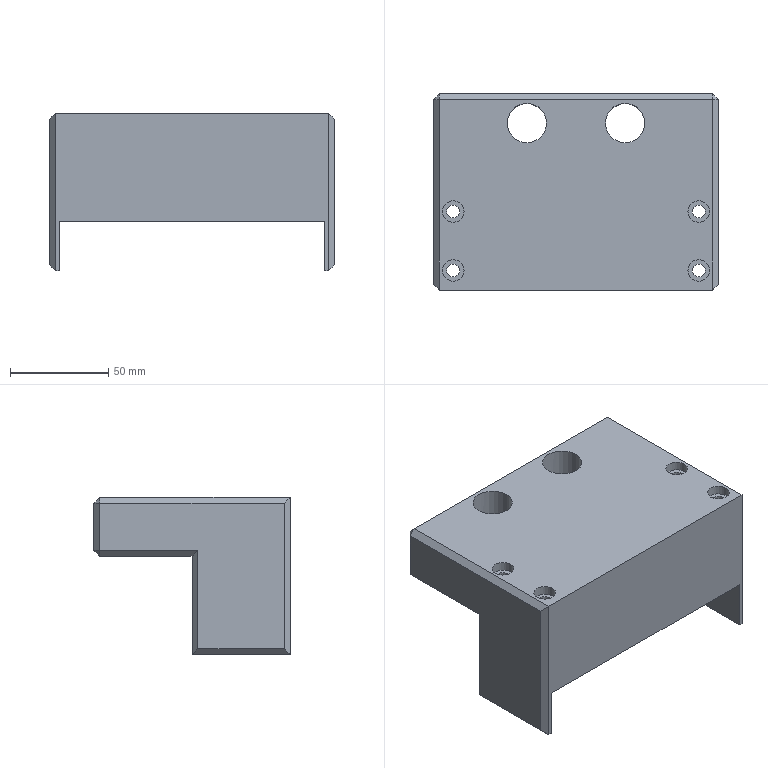NC program | NX | posted with a generic post | part box 145 x 100 x 80 mm
Lines 551 to 2025 of 2025, first 1325 of 1469 lines:
(ZLEVEL_PROFILE_1_COPY_1_COPY_COPY_1_COPY_COPY_COPY_COPY , TOOL : D8A45)
N1076 T06 M6
N1078 G54
N1080 G17 G0 G90 X-70.793 Y41.932 B0. C0. S7500 M3
N1082 G43 Z30. H6
N1084 Z-2.5
N1086 G94 G1 Z-3.5 F1000.
N1088 X-70.197 Y40.9
N1090 G3 X-69.504 Y40.5 R0.8
N1092 G1 X69.504
N1094 G2 X73. Y37.001 R3.504
N1096 G1 Y12.999
N1098 G2 X69.504 Y9.5 R3.498
N1100 G1 X-69.504
N1102 G2 X-73. Y12.999 R3.497
N1104 G1 Y37.001
N1106 G2 X-69.504 Y40.5 R3.504
N1108 G3 X-68.812 Y40.902 R0.8
N1110 G1 X-68.124 Y42.1
N1112 Z-2.5
N1114 G0 Z30.
(ZLEVEL_PROFILE_1_COPY_1_COPY_COPY_1_COPY_COPY_COPY_COPY_COPY , TOOL : D8A45)
N1116 X74.991 Y7.571
N1118 Z-52.5
N1120 G1 Z-53.5
N1122 X73.773 Y7.898
N1124 G3 X73. Y7.691 R0.8
N1126 G1 Y-37.002
N1128 Y-40.021
N1130 G2 X69.501 Y-43.5 R3.504
N1132 G1 X67.499
N1134 G2 X64. Y-40. R3.499
N1136 G1 Y-18.5
N1138 X-64.
N1140 Y-40.
N1142 G2 X-67.499 Y-43.5 R3.499
N1144 G1 X-69.501
N1146 G2 X-73. Y-40.021 R3.504
N1148 G1 Y-37.002
N1150 Y7.691
N1152 G3 X-73.773 Y7.898 R0.8
N1154 G1 X-74.991 Y7.571
N1156 Z-52.5
N1158 G0 Z30.
(ZLEVEL_PROFILE_1_COPY_1_COPY_COPY_1_COPY_COPY_COPY_COPY_COPY_COPY , TOOL : D8A45)
N1160 X-23.384 Y28.089
N1162 Z0.647
N1164 G1 Z-0.353
N1166 X-24.306 Y29.685
N1168 G3 X-24.999 Y30.085 R0.8
N1170 X-30.086 Y24.998 R5.087
N1172 X-24.999 Y30.085 R-5.087
N1174 G1 X-25.197 Y30.08 Z-0.357
N1176 X-25.395 Y30.065 Z-0.36
N1178 X-25.592 Y30.049 Z-0.364
N1180 X-25.69 Y30.031 Z-0.365
N1182 X-25.787 Y30.012 Z-0.367
N1184 X-26.175 Y29.935 Z-0.374
N1186 X-26.364 Y29.876 Z-0.377
N1188 X-26.552 Y29.815 Z-0.381
N1190 X-26.74 Y29.754 Z-0.384
N1192 X-26.831 Y29.715 Z-0.386
N1194 X-26.921 Y29.674 Z-0.388
N1196 X-27.278 Y29.509 Z-0.395
N1198 X-27.448 Y29.409 Z-0.398
N1200 X-27.616 Y29.306 Z-0.402
N1202 X-27.783 Y29.203 Z-0.405
N1204 X-27.941 Y29.084 Z-0.409
N1206 X-28.248 Y28.841 Z-0.416
N1208 X-28.389 Y28.704 Z-0.419
N1210 X-28.528 Y28.565 Z-0.423
N1212 X-28.666 Y28.427 Z-0.426
N1214 X-28.791 Y28.276 Z-0.429
N1216 X-29.032 Y27.969 Z-0.436
N1218 X-29.14 Y27.806 Z-0.44
N1220 X-29.241 Y27.639 Z-0.443
N1222 X-29.342 Y27.472 Z-0.447
N1224 X-29.43 Y27.298 Z-0.45
N1226 X-29.591 Y26.944 Z-0.457
N1228 X-29.659 Y26.762 Z-0.461
N1230 X-29.718 Y26.577 Z-0.464
N1232 X-29.777 Y26.392 Z-0.468
N1234 X-29.823 Y26.203 Z-0.471
N1236 X-29.896 Y25.822 Z-0.478
N1238 X-29.92 Y25.631 Z-0.481
N1240 X-29.934 Y25.437 Z-0.485
N1242 X-29.948 Y25.245 Z-0.488
N1244 X-29.95 Y25.051 Z-0.492
N1246 X-29.932 Y24.666 Z-0.499
N1248 X-29.913 Y24.474 Z-0.502
N1250 X-29.881 Y24.284 Z-0.506
N1252 X-29.849 Y24.094 Z-0.509
N1254 X-29.808 Y23.906 Z-0.513
N1256 X-29.7 Y23.537 Z-0.519
N1258 X-29.638 Y23.356 Z-0.523
N1260 X-29.563 Y23.179 Z-0.526
N1262 X-29.487 Y23.003 Z-0.53
N1264 X-29.405 Y22.83 Z-0.533
N1266 X-29.214 Y22.498 Z-0.54
N1268 X-29.113 Y22.336 Z-0.544
N1270 X-28.999 Y22.183 Z-0.547
N1272 X-28.885 Y22.03 Z-0.551
N1274 X-28.767 Y21.88 Z-0.554
N1276 X-28.504 Y21.604 Z-0.561
N1278 X-28.37 Y21.469 Z-0.564
N1280 X-28.223 Y21.348 Z-0.568
N1282 X-28.077 Y21.226 Z-0.571
N1284 X-27.929 Y21.108 Z-0.575
N1286 X-27.61 Y20.902 Z-0.582
N1288 X-27.449 Y20.801 Z-0.585
N1290 X-27.279 Y20.718 Z-0.589
N1292 X-27.109 Y20.635 Z-0.592
N1294 X-26.939 Y20.553 Z-0.596
N1296 X-26.582 Y20.428 Z-0.603
N1298 X-26.493 Y20.397 Z-0.604
N1300 X-26.404 Y20.367 Z-0.606
N1302 X-26.219 Y20.326 Z-0.61
N1304 X-26.035 Y20.285 Z-0.613
N1306 X-25.851 Y20.245 Z-0.616
N1308 X-25.477 Y20.207 Z-0.623
N1310 X-25.29 Y20.188 Z-0.627
N1312 X-25.196 Y20.189 Z-0.629
N1314 X-25.102 Y20.191 Z-0.63
N1316 X-24.727 Y20.198 Z-0.637
N1318 X-24.541 Y20.222 Z-0.641
N1320 X-24.356 Y20.248 Z-0.644
N1322 X-24.171 Y20.273 Z-0.648
N1324 X-23.989 Y20.318 Z-0.651
N1326 X-23.628 Y20.413 Z-0.658
N1328 X-23.453 Y20.478 Z-0.661
N1330 X-23.28 Y20.546 Z-0.665
N1332 X-23.106 Y20.614 Z-0.668
N1334 X-22.94 Y20.699 Z-0.672
N1336 X-22.613 Y20.874 Z-0.679
N1338 X-22.458 Y20.977 Z-0.682
N1340 X-22.306 Y21.083 Z-0.686
N1342 X-22.154 Y21.19 Z-0.689
N1344 X-22.012 Y21.309 Z-0.693
N1346 X-21.737 Y21.556 Z-0.7
N1348 X-21.61 Y21.69 Z-0.703
N1350 X-21.486 Y21.828 Z-0.706
N1352 G3 X-24.999 Y29.734 R4.734
N1354 G1 X-25.197 Y29.726 Z-0.71
N1356 X-25.394 Y29.711 Z-0.713
N1358 X-25.592 Y29.692 Z-0.717
N1360 X-25.786 Y29.653 Z-0.72
N1362 X-25.98 Y29.615 Z-0.724
N1364 X-26.172 Y29.569 Z-0.727
N1366 X-26.548 Y29.447 Z-0.734
N1368 X-26.731 Y29.375 Z-0.738
N1370 X-26.911 Y29.292 Z-0.741
N1372 X-27.089 Y29.21 Z-0.745
N1374 X-27.261 Y29.113 Z-0.748
N1376 X-27.596 Y28.907 Z-0.755
N1378 X-27.752 Y28.788 Z-0.758
N1380 X-27.906 Y28.666 Z-0.762
N1382 X-27.983 Y28.605 Z-0.764
N1384 X-28.058 Y28.543 Z-0.765
N1386 X-28.197 Y28.404 Z-0.769
N1388 X-28.335 Y28.265 Z-0.772
N1390 X-28.47 Y28.123 Z-0.776
N1392 X-28.711 Y27.815 Z-0.783
N1394 X-28.824 Y27.657 Z-0.786
N1396 X-28.925 Y27.49 Z-0.79
N1398 X-29.026 Y27.323 Z-0.793
N1400 X-29.117 Y27.151 Z-0.797
N1402 X-29.278 Y26.797 Z-0.803
N1404 X-29.343 Y26.614 Z-0.807
N1406 X-29.402 Y26.429 Z-0.81
N1408 X-29.461 Y26.244 Z-0.814
N1410 X-29.482 Y26.149 Z-0.816
N1412 X-29.5 Y26.054 Z-0.817
N1414 X-29.537 Y25.863 Z-0.821
N1416 X-29.572 Y25.673 Z-0.824
N1418 X-29.6 Y25.287 Z-0.831
N1420 X-29.609 Y25.094 Z-0.835
N1422 X-29.6 Y24.901 Z-0.838
N1424 X-29.59 Y24.709 Z-0.842
N1426 X-29.572 Y24.517 Z-0.845
N1428 X-29.509 Y24.137 Z-0.852
N1430 X-29.464 Y23.95 Z-0.855
N1432 X-29.41 Y23.765 Z-0.859
N1434 X-29.356 Y23.581 Z-0.862
N1436 X-29.287 Y23.402 Z-0.866
N1438 X-29.136 Y23.05 Z-0.873
N1440 X-29.043 Y22.883 Z-0.876
N1442 X-28.947 Y22.717 Z-0.88
N1444 X-28.9 Y22.634 Z-0.881
N1446 X-28.851 Y22.552 Z-0.883
N1448 X-28.736 Y22.398 Z-0.887
N1450 X-28.622 Y22.246 Z-0.89
N1452 X-28.504 Y22.096 Z-0.893
N1454 X-28.242 Y21.819 Z-0.9
N1456 X-28.104 Y21.688 Z-0.904
N1458 X-27.958 Y21.567 Z-0.907
N1460 X-27.812 Y21.445 Z-0.911
N1462 X-27.657 Y21.334 Z-0.914
N1464 X-27.339 Y21.128 Z-0.921
N1466 X-27.171 Y21.04 Z-0.925
N1468 X-27.001 Y20.957 Z-0.928
N1470 X-26.832 Y20.873 Z-0.932
N1472 X-26.743 Y20.841 Z-0.933
N1474 X-26.653 Y20.809 Z-0.935
N1476 X-26.475 Y20.747 Z-0.939
N1478 X-26.296 Y20.687 Z-0.942
N1480 X-25.928 Y20.605 Z-0.949
N1482 X-25.743 Y20.57 Z-0.952
N1484 X-25.556 Y20.551 Z-0.956
N1486 X-25.369 Y20.532 Z-0.959
N1488 X-25.181 Y20.524 Z-0.963
N1490 X-24.806 Y20.53 Z-0.97
N1492 X-24.62 Y20.548 Z-0.973
N1494 X-24.434 Y20.573 Z-0.977
N1496 X-24.249 Y20.599 Z-0.98
N1498 X-24.067 Y20.642 Z-0.984
N1500 X-23.705 Y20.736 Z-0.99
N1502 X-23.531 Y20.804 Z-0.994
N1504 X-23.358 Y20.872 Z-0.997
N1506 X-23.186 Y20.943 Z-1.001
N1508 X-23.021 Y21.031 Z-1.004
N1510 X-22.858 Y21.119 Z-1.008
N1512 X-22.697 Y21.213 Z-1.011
N1514 X-22.393 Y21.426 Z-1.018
N1516 X-22.248 Y21.54 Z-1.022
N1518 X-22.11 Y21.664 Z-1.025
N1520 X-21.972 Y21.787 Z-1.029
N1522 X-21.844 Y21.921 Z-1.032
N1524 X-21.6 Y22.198 Z-1.039
N1526 X-21.492 Y22.348 Z-1.042
N1528 X-21.387 Y22.5 Z-1.046
N1530 X-21.283 Y22.651 Z-1.049
N1532 X-21.24 Y22.733 Z-1.051
N1534 X-21.197 Y22.814 Z-1.053
N1536 X-21.111 Y22.977 Z-1.056
N1538 X-21.033 Y23.143 Z-1.06
N1540 G3 X-24.999 Y29.38 R4.381
N1542 G1 X-25.196 Y29.372 Z-1.063
N1544 X-25.393 Y29.357 Z-1.067
N1546 X-25.589 Y29.333 Z-1.071
N1548 X-25.782 Y29.294 Z-1.074
N1550 X-25.975 Y29.256 Z-1.078
N1552 X-26.164 Y29.201 Z-1.082
N1554 X-26.351 Y29.14 Z-1.085
N1556 X-26.537 Y29.076 Z-1.089
N1558 X-26.893 Y28.911 Z-1.097
N1560 X-27.066 Y28.819 Z-1.1
N1562 X-27.233 Y28.716 Z-1.104
N1564 X-27.399 Y28.614 Z-1.108
N1566 X-27.555 Y28.495 Z-1.111
N1568 X-27.708 Y28.373 Z-1.115
N1570 X-27.856 Y28.247 Z-1.119
N1572 X-28.131 Y27.97 Z-1.126
N1574 X-28.257 Y27.823 Z-1.13
N1576 X-28.377 Y27.67 Z-1.133
N1578 X-28.497 Y27.517 Z-1.137
N1580 X-28.548 Y27.434 Z-1.139
N1582 X-28.598 Y27.351 Z-1.141
N1584 X-28.698 Y27.185 Z-1.144
N1586 X-28.792 Y27.015 Z-1.148
N1588 X-28.952 Y26.663 Z-1.155
N1590 X-29.016 Y26.481 Z-1.159
N1592 X-29.075 Y26.297 Z-1.163
N1594 X-29.104 Y26.205 Z-1.165
N1596 X-29.131 Y26.113 Z-1.166
N1598 X-29.167 Y25.923 Z-1.17
N1600 X-29.204 Y25.734 Z-1.174
N1602 X-29.229 Y25.543 Z-1.177
N1604 X-29.256 Y25.16 Z-1.185
N1606 X-29.251 Y24.968 Z-1.189
N1608 X-29.242 Y24.776 Z-1.192
N1610 X-29.228 Y24.586 Z-1.196
N1612 X-29.196 Y24.396 Z-1.2
N1614 X-29.164 Y24.208 Z-1.203
N1616 X-29.12 Y24.022 Z-1.207
N1618 X-29.012 Y23.656 Z-1.214
N1620 X-28.938 Y23.48 Z-1.218
N1622 X-28.863 Y23.305 Z-1.222
N1624 X-28.782 Y23.133 Z-1.225
N1626 X-28.687 Y22.968 Z-1.229
N1628 X-28.592 Y22.804 Z-1.233
N1630 X-28.484 Y22.648 Z-1.236
N1632 X-28.371 Y22.496 Z-1.24
N1634 X-28.257 Y22.345 Z-1.244
N1636 X-27.996 Y22.07 Z-1.251
N1638 X-27.859 Y21.94 Z-1.255
N1640 X-27.714 Y21.82 Z-1.258
N1642 X-27.568 Y21.699 Z-1.262
N1644 X-27.412 Y21.593 Z-1.266
N1646 X-27.254 Y21.491 Z-1.269
N1648 X-27.094 Y21.392 Z-1.273
N1650 X-26.757 Y21.227 Z-1.281
N1652 X-26.583 Y21.156 Z-1.284
N1654 X-26.406 Y21.094 Z-1.288
N1656 X-26.23 Y21.032 Z-1.292
N1658 X-26.139 Y21.01 Z-1.293
N1660 X-26.047 Y20.99 Z-1.295
N1662 X-25.865 Y20.949 Z-1.299
N1664 X-25.681 Y20.915 Z-1.303
N1666 X-25.31 Y20.878 Z-1.31
N1668 X-25.123 Y20.874 Z-1.314
N1670 X-24.937 Y20.878 Z-1.317
N1672 X-24.844 Y20.88 Z-1.319
N1674 X-24.751 Y20.882 Z-1.321
N1676 X-24.567 Y20.908 Z-1.325
N1678 X-24.383 Y20.934 Z-1.328
N1680 X-24.201 Y20.968 Z-1.332
N1682 X-23.842 Y21.062 Z-1.339
N1684 X-23.669 Y21.125 Z-1.343
N1686 X-23.497 Y21.193 Z-1.347
N1688 X-23.326 Y21.263 Z-1.35
N1690 X-23.163 Y21.351 Z-1.354
N1692 X-23.001 Y21.438 Z-1.358
N1694 X-22.845 Y21.536 Z-1.361
N1696 X-22.544 Y21.747 Z-1.369
N1698 X-22.405 Y21.868 Z-1.372
N1700 X-22.269 Y21.991 Z-1.376
N1702 X-22.136 Y22.117 Z-1.38
N1704 X-22.015 Y22.255 Z-1.384
N1706 X-21.894 Y22.392 Z-1.387
N1708 X-21.784 Y22.538 Z-1.391
N1710 X-21.681 Y22.689 Z-1.395
N1712 X-21.577 Y22.839 Z-1.398
N1714 X-21.408 Y23.162 Z-1.406
N1716 X-21.33 Y23.327 Z-1.409
N1718 X-21.266 Y23.497 Z-1.413
N1720 G3 X-24.205 Y28.948 R4.025
N1722 X-24.999 Y29.027 R4.026
N1724 G1 X-25.195 Y29.018 Z-1.417
N1726 X-25.391 Y29.002 Z-1.421
N1728 X-25.585 Y28.973 Z-1.425
N1730 X-25.778 Y28.935 Z-1.429
N1732 X-25.969 Y28.893 Z-1.433
N1734 X-26.155 Y28.832 Z-1.437
N1736 X-26.341 Y28.771 Z-1.441
N1738 X-26.521 Y28.695 Z-1.445
N1740 X-26.698 Y28.612 Z-1.449
N1742 X-26.872 Y28.524 Z-1.453
N1744 X-27.037 Y28.422 Z-1.457
N1746 X-27.203 Y28.319 Z-1.461
N1748 X-27.357 Y28.201 Z-1.465
N1750 X-27.509 Y28.08 Z-1.469
N1752 X-27.653 Y27.95 Z-1.473
N1754 X-27.79 Y27.812 Z-1.477
N1756 X-27.857 Y27.743 Z-1.479
N1758 X-27.925 Y27.674 Z-1.481
N1760 X-27.985 Y27.598 Z-1.483
N1762 X-28.045 Y27.522 Z-1.485
N1764 X-28.163 Y27.369 Z-1.489
N1766 X-28.271 Y27.209 Z-1.493
N1768 X-28.37 Y27.044 Z-1.497
N1770 X-28.467 Y26.877 Z-1.501
N1772 X-28.546 Y26.702 Z-1.505
N1774 X-28.625 Y26.527 Z-1.509
N1776 X-28.688 Y26.345 Z-1.513
N1778 X-28.746 Y26.162 Z-1.517
N1780 X-28.797 Y25.978 Z-1.521
N1782 X-28.833 Y25.789 Z-1.525
N1784 X-28.868 Y25.602 Z-1.529
N1786 X-28.884 Y25.411 Z-1.533
N1788 X-28.897 Y25.221 Z-1.537
N1790 X-28.9 Y25.03 Z-1.541
N1792 X-28.89 Y24.84 Z-1.545
N1794 X-28.88 Y24.649 Z-1.549
N1796 X-28.848 Y24.462 Z-1.553
N1798 X-28.816 Y24.275 Z-1.557
N1800 X-28.771 Y24.091 Z-1.561
N1802 X-28.717 Y23.909 Z-1.566
N1804 X-28.66 Y23.728 Z-1.57
N1806 X-28.585 Y23.554 Z-1.574
N1808 X-28.51 Y23.381 Z-1.578
N1810 X-28.421 Y23.214 Z-1.582
N1812 X-28.326 Y23.052 Z-1.586
N1814 X-28.226 Y22.892 Z-1.59
N1816 X-28.112 Y22.742 Z-1.594
N1818 X-28. Y22.591 Z-1.598
N1820 X-27.871 Y22.454 Z-1.602
N1822 X-27.742 Y22.318 Z-1.606
N1824 X-27.605 Y22.19 Z-1.61
N1826 X-27.461 Y22.07 Z-1.614
N1828 X-27.388 Y22.011 Z-1.616
N1830 X-27.316 Y21.952 Z-1.618
N1832 X-27.237 Y21.902 Z-1.62
N1834 X-27.158 Y21.851 Z-1.622
N1836 X-27.001 Y21.75 Z-1.626
N1838 X-26.838 Y21.661 Z-1.63
N1840 X-26.67 Y21.58 Z-1.634
N1842 X-26.501 Y21.502 Z-1.638
N1844 X-26.325 Y21.441 Z-1.642
N1846 X-26.15 Y21.38 Z-1.646
N1848 X-25.97 Y21.336 Z-1.65
N1850 X-25.788 Y21.296 Z-1.654
N1852 X-25.606 Y21.264 Z-1.658
N1854 X-25.422 Y21.246 Z-1.662
N1856 X-25.238 Y21.228 Z-1.666
N1858 X-25.053 Y21.23 Z-1.67
N1860 X-24.869 Y21.235 Z-1.674
N1862 X-24.685 Y21.249 Z-1.678
N1864 X-24.504 Y21.275 Z-1.682
N1866 X-24.322 Y21.302 Z-1.686
N1868 X-24.144 Y21.35 Z-1.69
N1870 X-23.967 Y21.396 Z-1.694
N1872 X-23.794 Y21.457 Z-1.698
N1874 X-23.624 Y21.524 Z-1.702
N1876 X-23.456 Y21.596 Z-1.706
N1878 X-23.295 Y21.683 Z-1.71
N1880 X-23.135 Y21.77 Z-1.714
N1882 X-22.983 Y21.871 Z-1.718
N1884 X-22.835 Y21.977 Z-1.722
N1886 X-22.691 Y22.088 Z-1.726
N1888 X-22.557 Y22.21 Z-1.73
N1890 X-22.421 Y22.331 Z-1.734
N1892 X-22.302 Y22.467 Z-1.738
N1894 X-22.182 Y22.603 Z-1.742
N1896 X-22.072 Y22.746 Z-1.746
N1898 X-21.97 Y22.895 Z-1.75
N1900 X-21.87 Y23.045 Z-1.754
N1902 X-21.786 Y23.205 Z-1.758
N1904 X-21.703 Y23.365 Z-1.762
N1906 X-21.633 Y23.53 Z-1.766
N1908 G3 X-24.999 Y28.673 R3.674
N1910 G1 X-25.194 Y28.664 Z-1.771
N1912 X-25.389 Y28.649 Z-1.775
N1914 X-25.581 Y28.614 Z-1.779
N1916 X-25.772 Y28.576 Z-1.784
N1918 X-25.959 Y28.525 Z-1.788
N1920 X-26.144 Y28.464 Z-1.793
N1922 X-26.326 Y28.396 Z-1.797
N1924 X-26.502 Y28.315 Z-1.802
N1926 X-26.676 Y28.23 Z-1.806
N1928 X-26.841 Y28.128 Z-1.81
N1930 X-27.004 Y28.026 Z-1.815
N1932 X-27.158 Y27.908 Z-1.819
N1934 X-27.307 Y27.788 Z-1.824
N1936 X-27.448 Y27.656 Z-1.828
N1938 X-27.582 Y27.518 Z-1.832
N1940 X-27.711 Y27.376 Z-1.837
N1942 X-27.827 Y27.224 Z-1.841
N1944 X-27.942 Y27.071 Z-1.846
N1946 X-28.04 Y26.906 Z-1.85
N1948 X-28.139 Y26.743 Z-1.855
N1950 X-28.217 Y26.569 Z-1.859
N1952 X-28.296 Y26.395 Z-1.863
N1954 X-28.358 Y26.215 Z-1.868
N1956 X-28.416 Y26.034 Z-1.872
N1958 X-28.461 Y25.85 Z-1.877
N1960 X-28.497 Y25.664 Z-1.881
N1962 X-28.525 Y25.477 Z-1.885
N1964 X-28.538 Y25.288 Z-1.89
N1966 X-28.549 Y25.1 Z-1.894
N1968 X-28.54 Y24.911 Z-1.899
N1970 X-28.529 Y24.723 Z-1.903
N1972 X-28.502 Y24.536 Z-1.908
N1974 X-28.469 Y24.352 Z-1.912
N1976 X-28.426 Y24.169 Z-1.916
N1978 X-28.371 Y23.99 Z-1.921
N1980 X-28.311 Y23.812 Z-1.925
N1982 X-28.236 Y23.641 Z-1.93
N1984 X-28.16 Y23.47 Z-1.934
N1986 X-28.066 Y23.31 Z-1.938
N1988 X-27.973 Y23.148 Z-1.943
N1990 X-27.862 Y22.998 Z-1.947
N1992 X-27.751 Y22.849 Z-1.952
N1994 X-27.627 Y22.711 Z-1.956
N1996 X-27.499 Y22.577 Z-1.96
N1998 X-27.364 Y22.451 Z-1.965
N2000 X-27.222 Y22.332 Z-1.969
N2002 X-27.076 Y22.22 Z-1.974
N2004 X-26.921 Y22.119 Z-1.978
N2006 X-26.765 Y22.021 Z-1.983
N2008 X-26.6 Y21.939 Z-1.987
N2010 X-26.435 Y21.86 Z-1.991
N2012 X-26.263 Y21.794 Z-1.996
N2014 X-26.09 Y21.736 Z-2.
N2016 X-25.914 Y21.686 Z-2.005
N2018 X-25.735 Y21.648 Z-2.009
N2020 X-25.555 Y21.615 Z-2.013
N2022 X-25.374 Y21.598 Z-2.018
N2024 X-25.192 Y21.582 Z-2.022
N2026 X-25.011 Y21.587 Z-2.027
N2028 X-24.829 Y21.59 Z-2.031
N2030 X-24.649 Y21.613 Z-2.036
N2032 X-24.47 Y21.638 Z-2.04
N2034 X-24.293 Y21.678 Z-2.044
N2036 X-24.118 Y21.723 Z-2.049
N2038 X-23.947 Y21.779 Z-2.053
N2040 X-23.779 Y21.845 Z-2.058
N2042 X-23.614 Y21.915 Z-2.062
N2044 X-23.455 Y22. Z-2.066
N2046 X-23.298 Y22.087 Z-2.071
N2048 X-23.15 Y22.188 Z-2.075
N2050 X-23.005 Y22.293 Z-2.08
N2052 X-22.867 Y22.407 Z-2.084
N2054 X-22.736 Y22.527 Z-2.089
N2056 X-22.609 Y22.654 Z-2.093
N2058 X-22.493 Y22.788 Z-2.097
N2060 X-22.379 Y22.925 Z-2.102
N2062 X-22.28 Y23.072 Z-2.106
N2064 X-22.18 Y23.219 Z-2.111
N2066 X-22.099 Y23.376 Z-2.115
N2068 X-22.023 Y23.536 Z-2.119
N2070 G3 X-24.999 Y28.32 R3.318
N2072 G1 X-25.193 Y28.31 Z-2.124
N2074 X-25.387 Y28.295 Z-2.129
N2076 X-25.578 Y28.255 Z-2.134
N2078 X-25.768 Y28.217 Z-2.139
N2080 X-25.952 Y28.156 Z-2.143
N2082 X-26.136 Y28.096 Z-2.148
N2084 X-26.311 Y28.014 Z-2.153
N2086 X-26.486 Y27.933 Z-2.158
N2088 X-26.65 Y27.832 Z-2.163
N2090 X-26.814 Y27.731 Z-2.167
N2092 X-26.964 Y27.612 Z-2.172
N2094 X-27.115 Y27.492 Z-2.177
N2096 X-27.249 Y27.356 Z-2.182
N2098 X-27.384 Y27.22 Z-2.187
N2100 X-27.502 Y27.071 Z-2.191
N2102 X-27.619 Y26.92 Z-2.196
N2104 X-27.72 Y26.758 Z-2.201
N2106 X-27.818 Y26.595 Z-2.206
N2108 X-27.898 Y26.424 Z-2.211
N2110 X-27.976 Y26.251 Z-2.215
N2112 X-28.036 Y26.071 Z-2.22
N2114 X-28.093 Y25.891 Z-2.225
N2116 X-28.132 Y25.706 Z-2.23
N2118 X-28.167 Y25.521 Z-2.235
N2120 X-28.183 Y25.334 Z-2.239
N2122 X-28.196 Y25.146 Z-2.244
N2124 X-28.191 Y24.959 Z-2.249
N2126 X-28.182 Y24.771 Z-2.254
N2128 X-28.155 Y24.586 Z-2.258
N2130 X-28.123 Y24.402 Z-2.263
N2132 X-28.076 Y24.222 Z-2.268
N2134 X-28.023 Y24.043 Z-2.273
N2136 X-27.955 Y23.87 Z-2.278
N2138 X-27.881 Y23.7 Z-2.282
N2140 X-27.794 Y23.536 Z-2.287
N2142 X-27.701 Y23.376 Z-2.292
N2144 X-27.595 Y23.224 Z-2.297
N2146 X-27.484 Y23.077 Z-2.302
N2148 X-27.362 Y22.939 Z-2.306
N2150 X-27.235 Y22.806 Z-2.311
N2152 X-27.098 Y22.683 Z-2.316
N2154 X-26.956 Y22.566 Z-2.321
N2156 X-26.807 Y22.461 Z-2.326
N2158 X-26.652 Y22.362 Z-2.33
N2160 X-26.492 Y22.275 Z-2.335
N2162 X-26.328 Y22.195 Z-2.34
N2164 X-26.159 Y22.128 Z-2.345
N2166 X-25.987 Y22.068 Z-2.35
N2168 X-25.812 Y22.021 Z-2.354
N2170 X-25.634 Y21.982 Z-2.359
N2172 X-25.455 Y21.955 Z-2.364
N2174 X-25.275 Y21.938 Z-2.369
N2176 X-25.095 Y21.932 Z-2.374
N2178 X-24.915 Y21.937 Z-2.378
N2180 X-24.736 Y21.952 Z-2.383
N2182 X-24.558 Y21.977 Z-2.388
N2184 X-24.382 Y22.013 Z-2.393
N2186 X-24.209 Y22.059 Z-2.397
N2188 X-24.039 Y22.115 Z-2.402
N2190 X-23.873 Y22.181 Z-2.407
N2192 X-23.712 Y22.256 Z-2.412
N2194 X-23.555 Y22.341 Z-2.417
N2196 X-23.404 Y22.434 Z-2.421
N2198 X-23.259 Y22.537 Z-2.426
N2200 X-23.12 Y22.646 Z-2.431
N2202 X-22.989 Y22.765 Z-2.436
N2204 X-22.864 Y22.889 Z-2.441
N2206 X-22.748 Y23.022 Z-2.445
N2208 X-22.639 Y23.16 Z-2.45
N2210 X-22.54 Y23.305 Z-2.455
N2212 X-22.448 Y23.454 Z-2.46
N2214 X-22.369 Y23.611 Z-2.465
N2216 G3 X-24.999 Y27.975 R2.975
N2218 G1 X-25.192 Y27.965 Z-2.47
N2220 X-25.385 Y27.945 Z-2.475
N2222 X-25.574 Y27.905 Z-2.481
N2224 X-25.761 Y27.858 Z-2.486
N2226 X-25.943 Y27.797 Z-2.492
N2228 X-26.122 Y27.724 Z-2.497
N2230 X-26.295 Y27.642 Z-2.502
N2232 X-26.46 Y27.545 Z-2.508
N2234 X-26.541 Y27.494 Z-2.51
N2236 X-26.622 Y27.444 Z-2.513
N2238 X-26.698 Y27.385 Z-2.516
N2240 X-26.772 Y27.325 Z-2.519
N2242 X-26.918 Y27.203 Z-2.524
N2244 X-27.051 Y27.067 Z-2.529
N2246 X-27.179 Y26.927 Z-2.535
N2248 X-27.294 Y26.777 Z-2.54
N2250 X-27.401 Y26.621 Z-2.545
N2252 X-27.497 Y26.459 Z-2.551
N2254 X-27.581 Y26.29 Z-2.556
N2256 X-27.657 Y26.118 Z-2.562
N2258 X-27.716 Y25.94 Z-2.567
N2260 X-27.771 Y25.761 Z-2.572
N2262 X-27.805 Y25.577 Z-2.578
N2264 X-27.835 Y25.393 Z-2.583
N2266 X-27.846 Y25.207 Z-2.589
N2268 X-27.85 Y25.021 Z-2.594
N2270 X-27.839 Y24.836 Z-2.599
N2272 X-27.816 Y24.652 Z-2.605
N2274 X-27.784 Y24.47 Z-2.61
N2276 X-27.736 Y24.292 Z-2.616
N2278 X-27.683 Y24.116 Z-2.621
N2280 X-27.611 Y23.946 Z-2.626
N2282 X-27.574 Y23.862 Z-2.629
N2284 X-27.536 Y23.779 Z-2.632
N2286 X-27.489 Y23.7 Z-2.634
N2288 X-27.443 Y23.621 Z-2.637
N2290 X-27.346 Y23.467 Z-2.643
N2292 X-27.235 Y23.321 Z-2.648
N2294 X-27.117 Y23.183 Z-2.653
N2296 X-26.991 Y23.052 Z-2.659
N2298 X-26.856 Y22.931 Z-2.664
N2300 X-26.715 Y22.817 Z-2.67
N2302 X-26.565 Y22.717 Z-2.675
N2304 X-26.412 Y22.621 Z-2.68
N2306 X-26.25 Y22.543 Z-2.686
N2308 X-26.086 Y22.468 Z-2.691
N2310 X-25.917 Y22.411 Z-2.696
N2312 X-25.745 Y22.36 Z-2.702
N2314 X-25.57 Y22.324 Z-2.707
N2316 X-25.394 Y22.297 Z-2.713
N2318 X-25.217 Y22.282 Z-2.718
N2320 X-25.039 Y22.281 Z-2.723
N2322 X-24.862 Y22.286 Z-2.729
N2324 X-24.686 Y22.31 Z-2.734
N2326 X-24.512 Y22.337 Z-2.74
N2328 X-24.342 Y22.383 Z-2.745
N2330 X-24.174 Y22.434 Z-2.75
N2332 X-24.011 Y22.501 Z-2.756
N2334 X-23.853 Y22.574 Z-2.761
N2336 X-23.7 Y22.659 Z-2.767
N2338 X-23.554 Y22.754 Z-2.772
N2340 X-23.412 Y22.855 Z-2.777
N2342 X-23.281 Y22.969 Z-2.783
N2344 X-23.154 Y23.087 Z-2.788
N2346 X-23.04 Y23.217 Z-2.794
N2348 X-22.93 Y23.35 Z-2.799
N2350 X-22.834 Y23.493 Z-2.804
N2352 X-22.745 Y23.64 Z-2.81
N2354 G3 X-24.999 Y27.633 R2.633
N2356 G1 X-25.198 Y27.62 Z-2.816
N2358 X-25.396 Y27.593 Z-2.823
N2360 X-25.59 Y27.55 Z-2.829
N2362 X-25.779 Y27.49 Z-2.835
N2364 X-25.964 Y27.419 Z-2.842
N2366 X-26.142 Y27.334 Z-2.848
N2368 X-26.311 Y27.233 Z-2.854
N2370 X-26.475 Y27.124 Z-2.861
N2372 X-26.626 Y27. Z-2.867
N2374 X-26.769 Y26.865 Z-2.874
N2376 X-26.902 Y26.723 Z-2.88
N2378 X-27.021 Y26.569 Z-2.886
N2380 X-27.128 Y26.407 Z-2.893
N2382 X-27.227 Y26.24 Z-2.899
N2384 X-27.304 Y26.064 Z-2.906
N2386 X-27.374 Y25.884 Z-2.912
N2388 X-27.429 Y25.7 Z-2.918
N2390 X-27.467 Y25.512 Z-2.925
N2392 X-27.493 Y25.323 Z-2.931
N2394 X-27.505 Y25.132 Z-2.938
N2396 X-27.499 Y24.942 Z-2.944
N2398 X-27.485 Y24.753 Z-2.95
N2400 X-27.45 Y24.567 Z-2.957
N2402 X-27.404 Y24.384 Z-2.963
N2404 X-27.347 Y24.205 Z-2.97
N2406 X-27.272 Y24.032 Z-2.976
N2408 X-27.186 Y23.866 Z-2.982
N2410 X-27.091 Y23.705 Z-2.989
N2412 X-26.978 Y23.556 Z-2.995
N2414 X-26.86 Y23.413 Z-3.001
N2416 X-26.73 Y23.281 Z-3.008
N2418 X-26.589 Y23.16 Z-3.014
N2420 X-26.442 Y23.049 Z-3.021
N2422 X-26.287 Y22.951 Z-3.027
N2424 X-26.124 Y22.867 Z-3.033
N2426 X-25.958 Y22.789 Z-3.04
N2428 X-25.784 Y22.733 Z-3.046
N2430 X-25.608 Y22.685 Z-3.053
N2432 X-25.431 Y22.65 Z-3.059
N2434 X-25.25 Y22.632 Z-3.065
N2436 X-25.07 Y22.627 Z-3.072
N2438 X-24.889 Y22.632 Z-3.078
N2440 X-24.712 Y22.658 Z-3.085
N2442 X-24.535 Y22.689 Z-3.091
N2444 X-24.364 Y22.739 Z-3.097
N2446 X-24.196 Y22.8 Z-3.104
N2448 X-24.034 Y22.872 Z-3.11
N2450 X-23.878 Y22.957 Z-3.117
N2452 X-23.731 Y23.055 Z-3.123
N2454 X-23.588 Y23.158 Z-3.129
N2456 X-23.46 Y23.279 Z-3.136
N2458 X-23.337 Y23.404 Z-3.142
N2460 X-23.225 Y23.538 Z-3.148
N2462 X-23.126 Y23.682 Z-3.155
N2464 G3 X-22.744 Y24.602 R2.287
N2466 X-24.999 Y27.291 R2.29
N2468 G1 X-25.198 Y27.275 Z-3.162
N2470 X-25.394 Y27.241 Z-3.17
N2472 X-25.586 Y27.192 Z-3.177
N2474 X-25.773 Y27.127 Z-3.185
N2476 X-25.951 Y27.043 Z-3.192
N2478 X-26.122 Y26.945 Z-3.2
N2480 X-26.284 Y26.836 Z-3.207
N2482 X-26.435 Y26.711 Z-3.215
N2484 X-26.57 Y26.573 Z-3.222
N2486 X-26.696 Y26.424 Z-3.23
N2488 X-26.754 Y26.347 Z-3.234
N2490 X-26.81 Y26.269 Z-3.237
N2492 X-26.858 Y26.185 Z-3.241
N2494 X-26.906 Y26.102 Z-3.245
N2496 X-26.987 Y25.928 Z-3.252
N2498 X-27.054 Y25.748 Z-3.26
N2500 X-27.081 Y25.657 Z-3.264
N2502 X-27.106 Y25.566 Z-3.267
N2504 X-27.122 Y25.472 Z-3.271
N2506 X-27.138 Y25.378 Z-3.275
N2508 X-27.154 Y25.19 Z-3.282
N2510 X-27.156 Y25.001 Z-3.29
N2512 X-27.15 Y24.907 Z-3.294
N2514 X-27.143 Y24.814 Z-3.297
N2516 X-27.126 Y24.721 Z-3.301
N2518 X-27.109 Y24.629 Z-3.305
N2520 X-27.061 Y24.449 Z-3.312
N2522 X-26.999 Y24.273 Z-3.32
N2524 X-26.923 Y24.104 Z-3.327
N2526 X-26.829 Y23.944 Z-3.335
N2528 X-26.724 Y23.794 Z-3.342
N2530 X-26.608 Y23.651 Z-3.35
N2532 X-26.48 Y23.521 Z-3.357
N2534 X-26.339 Y23.404 Z-3.365
N2536 X-26.191 Y23.3 Z-3.372
N2538 X-26.036 Y23.206 Z-3.38
N2540 X-25.864 Y23.13 Z-3.388
N2542 X-25.703 Y23.069 Z-3.395
N2544 X-25.509 Y23.021 Z-3.403
N2546 X-25.354 Y22.989 Z-3.41
N2548 X-25.168 Y22.977 Z-3.418
N2550 X-25. Y22.973 Z-3.425
N2552 X-24.816 Y22.994 Z-3.433
N2554 X-24.65 Y23.018 Z-3.44
N2556 X-24.476 Y23.07 Z-3.448
N2558 X-24.316 Y23.122 Z-3.455
N2560 X-24.006 Y23.279 Z-3.47
N2562 X-23.733 Y23.491 Z-3.485
N2564 X-23.612 Y23.612 Z-3.492
N2566 X-23.505 Y23.746 Z-3.5
N2568 G3 X-23.302 Y24.036 R1.979
N2570 X-24.602 Y23.088 R-1.951
N2572 X-23.505 Y23.746 R1.979
N2574 X-23.364 Y24.534 R0.8
N2576 G1 X-24.661 Y24.903
N2578 Z-2.5
N2580 G0 Z30.
N2582 X26.616 Y28.089
N2584 Z0.647
N2586 G1 Z-0.353
N2588 X25.694 Y29.685
N2590 G3 X25.001 Y30.085 R0.8
N2592 X19.914 Y24.998 R5.087
N2594 X25.001 Y30.085 R-5.087
N2596 G1 X24.803 Y30.08 Z-0.357
N2598 X24.605 Y30.065 Z-0.36
N2600 X24.408 Y30.049 Z-0.364
N2602 X24.31 Y30.031 Z-0.365
N2604 X24.213 Y30.012 Z-0.367
N2606 X23.825 Y29.935 Z-0.374
N2608 X23.636 Y29.876 Z-0.377
N2610 X23.448 Y29.815 Z-0.381
N2612 X23.26 Y29.754 Z-0.384
N2614 X23.169 Y29.715 Z-0.386
N2616 X23.079 Y29.674 Z-0.388
N2618 X22.722 Y29.509 Z-0.395
N2620 X22.552 Y29.409 Z-0.398
N2622 X22.384 Y29.306 Z-0.402
N2624 X22.217 Y29.203 Z-0.405
N2626 X22.059 Y29.084 Z-0.409
N2628 X21.752 Y28.841 Z-0.416
N2630 X21.611 Y28.704 Z-0.419
N2632 X21.472 Y28.565 Z-0.423
N2634 X21.334 Y28.427 Z-0.426
N2636 X21.209 Y28.276 Z-0.429
N2638 X20.968 Y27.969 Z-0.436
N2640 X20.86 Y27.806 Z-0.44
N2642 X20.759 Y27.639 Z-0.443
N2644 X20.658 Y27.472 Z-0.447
N2646 X20.57 Y27.298 Z-0.45
N2648 X20.409 Y26.944 Z-0.457
N2650 X20.341 Y26.762 Z-0.461
N2652 X20.282 Y26.577 Z-0.464
N2654 X20.223 Y26.392 Z-0.468
N2656 X20.177 Y26.203 Z-0.471
N2658 X20.104 Y25.822 Z-0.478
N2660 X20.08 Y25.631 Z-0.481
N2662 X20.066 Y25.437 Z-0.485
N2664 X20.052 Y25.245 Z-0.488
N2666 X20.05 Y25.051 Z-0.492
N2668 X20.068 Y24.666 Z-0.499
N2670 X20.087 Y24.474 Z-0.502
N2672 X20.119 Y24.284 Z-0.506
N2674 X20.151 Y24.094 Z-0.509
N2676 X20.192 Y23.906 Z-0.513
N2678 X20.3 Y23.537 Z-0.519
N2680 X20.362 Y23.356 Z-0.523
N2682 X20.437 Y23.179 Z-0.526
N2684 X20.513 Y23.003 Z-0.53
N2686 X20.595 Y22.83 Z-0.533
N2688 X20.786 Y22.498 Z-0.54
N2690 X20.887 Y22.336 Z-0.544
N2692 X21.001 Y22.183 Z-0.547
N2694 X21.115 Y22.03 Z-0.551
N2696 X21.233 Y21.88 Z-0.554
N2698 X21.496 Y21.604 Z-0.561
N2700 X21.63 Y21.469 Z-0.564
N2702 X21.777 Y21.348 Z-0.568
N2704 X21.923 Y21.226 Z-0.571
N2706 X22.071 Y21.108 Z-0.575
N2708 X22.39 Y20.902 Z-0.582
N2710 X22.551 Y20.801 Z-0.585
N2712 X22.721 Y20.718 Z-0.589
N2714 X22.891 Y20.635 Z-0.592
N2716 X23.061 Y20.553 Z-0.596
N2718 X23.418 Y20.428 Z-0.603
N2720 X23.507 Y20.397 Z-0.604
N2722 X23.596 Y20.367 Z-0.606
N2724 X23.781 Y20.326 Z-0.61
N2726 X23.965 Y20.285 Z-0.613
N2728 X24.149 Y20.245 Z-0.616
N2730 X24.523 Y20.207 Z-0.623
N2732 X24.71 Y20.188 Z-0.627
N2734 X24.804 Y20.189 Z-0.629
N2736 X24.898 Y20.191 Z-0.63
N2738 X25.273 Y20.198 Z-0.637
N2740 X25.459 Y20.222 Z-0.641
N2742 X25.644 Y20.248 Z-0.644
N2744 X25.829 Y20.273 Z-0.648
N2746 X26.011 Y20.318 Z-0.651
N2748 X26.372 Y20.413 Z-0.658
N2750 X26.547 Y20.478 Z-0.661
N2752 X26.72 Y20.546 Z-0.665
N2754 X26.894 Y20.614 Z-0.668
N2756 X27.06 Y20.699 Z-0.672
N2758 X27.387 Y20.874 Z-0.679
N2760 X27.542 Y20.977 Z-0.682
N2762 X27.694 Y21.083 Z-0.686
N2764 X27.846 Y21.19 Z-0.689
N2766 X27.988 Y21.309 Z-0.693
N2768 X28.263 Y21.556 Z-0.7
N2770 X28.39 Y21.69 Z-0.703
N2772 X28.514 Y21.828 Z-0.706
N2774 G3 X25.001 Y29.734 R4.734
N2776 G1 X24.803 Y29.726 Z-0.71
N2778 X24.606 Y29.711 Z-0.713
N2780 X24.408 Y29.692 Z-0.717
N2782 X24.214 Y29.653 Z-0.72
N2784 X24.02 Y29.615 Z-0.724
N2786 X23.828 Y29.569 Z-0.727
N2788 X23.452 Y29.447 Z-0.734
N2790 X23.269 Y29.375 Z-0.738
N2792 X23.089 Y29.292 Z-0.741
N2794 X22.911 Y29.21 Z-0.745
N2796 X22.739 Y29.113 Z-0.748
N2798 X22.404 Y28.907 Z-0.755
N2800 X22.248 Y28.788 Z-0.758
N2802 X22.094 Y28.666 Z-0.762
N2804 X22.017 Y28.605 Z-0.764
N2806 X21.942 Y28.543 Z-0.765
N2808 X21.803 Y28.404 Z-0.769
N2810 X21.665 Y28.265 Z-0.772
N2812 X21.53 Y28.123 Z-0.776
N2814 X21.289 Y27.815 Z-0.783
N2816 X21.176 Y27.657 Z-0.786
N2818 X21.075 Y27.49 Z-0.79
N2820 X20.974 Y27.323 Z-0.793
N2822 X20.883 Y27.151 Z-0.797
N2824 X20.722 Y26.797 Z-0.803
N2826 X20.657 Y26.614 Z-0.807
N2828 X20.598 Y26.429 Z-0.81
N2830 X20.539 Y26.244 Z-0.814
N2832 X20.518 Y26.149 Z-0.816
N2834 X20.5 Y26.054 Z-0.817
N2836 X20.463 Y25.863 Z-0.821
N2838 X20.428 Y25.673 Z-0.824
N2840 X20.4 Y25.287 Z-0.831
N2842 X20.391 Y25.094 Z-0.835
N2844 X20.4 Y24.901 Z-0.838
N2846 X20.41 Y24.709 Z-0.842
N2848 X20.428 Y24.517 Z-0.845
N2850 X20.491 Y24.137 Z-0.852
N2852 X20.536 Y23.95 Z-0.855
N2854 X20.59 Y23.765 Z-0.859
N2856 X20.644 Y23.581 Z-0.862
N2858 X20.713 Y23.402 Z-0.866
N2860 X20.864 Y23.05 Z-0.873
N2862 X20.957 Y22.883 Z-0.876
N2864 X21.053 Y22.717 Z-0.88
N2866 X21.1 Y22.634 Z-0.881
N2868 X21.149 Y22.552 Z-0.883
N2870 X21.264 Y22.398 Z-0.887
N2872 X21.378 Y22.246 Z-0.89
N2874 X21.496 Y22.096 Z-0.893
N2876 X21.758 Y21.819 Z-0.9
N2878 X21.896 Y21.688 Z-0.904
N2880 X22.042 Y21.567 Z-0.907
N2882 X22.188 Y21.445 Z-0.911
N2884 X22.343 Y21.334 Z-0.914
N2886 X22.661 Y21.128 Z-0.921
N2888 X22.829 Y21.04 Z-0.925
N2890 X22.999 Y20.957 Z-0.928
N2892 X23.168 Y20.873 Z-0.932
N2894 X23.257 Y20.841 Z-0.933
N2896 X23.347 Y20.809 Z-0.935
N2898 X23.525 Y20.747 Z-0.939
N2900 X23.704 Y20.687 Z-0.942
N2902 X24.072 Y20.605 Z-0.949
N2904 X24.257 Y20.57 Z-0.952
N2906 X24.444 Y20.551 Z-0.956
N2908 X24.631 Y20.532 Z-0.959
N2910 X24.819 Y20.524 Z-0.963
N2912 X25.194 Y20.53 Z-0.97
N2914 X25.38 Y20.548 Z-0.973
N2916 X25.566 Y20.573 Z-0.977
N2918 X25.751 Y20.599 Z-0.98
N2920 X25.933 Y20.642 Z-0.984
N2922 X26.295 Y20.736 Z-0.99
N2924 X26.469 Y20.804 Z-0.994
N2926 X26.642 Y20.872 Z-0.997
N2928 X26.814 Y20.943 Z-1.001
N2930 X26.979 Y21.031 Z-1.004
N2932 X27.142 Y21.119 Z-1.008
N2934 X27.303 Y21.213 Z-1.011
N2936 X27.607 Y21.426 Z-1.018
N2938 X27.752 Y21.54 Z-1.022
N2940 X27.89 Y21.664 Z-1.025
N2942 X28.028 Y21.787 Z-1.029
N2944 X28.156 Y21.921 Z-1.032
N2946 X28.4 Y22.198 Z-1.039
N2948 X28.508 Y22.348 Z-1.042
N2950 X28.613 Y22.5 Z-1.046
N2952 X28.717 Y22.651 Z-1.049
N2954 X28.76 Y22.733 Z-1.051
N2956 X28.803 Y22.814 Z-1.053
N2958 X28.889 Y22.977 Z-1.056
N2960 X28.967 Y23.143 Z-1.06
N2962 G3 X25.001 Y29.38 R4.381
N2964 G1 X24.804 Y29.372 Z-1.063
N2966 X24.607 Y29.357 Z-1.067
N2968 X24.411 Y29.333 Z-1.071
N2970 X24.218 Y29.294 Z-1.074
N2972 X24.025 Y29.256 Z-1.078
N2974 X23.836 Y29.201 Z-1.082
N2976 X23.649 Y29.14 Z-1.085
N2978 X23.463 Y29.076 Z-1.089
N2980 X23.107 Y28.911 Z-1.097
N2982 X22.934 Y28.819 Z-1.1
N2984 X22.767 Y28.716 Z-1.104
N2986 X22.601 Y28.614 Z-1.108
N2988 X22.445 Y28.495 Z-1.111
N2990 X22.292 Y28.373 Z-1.115
N2992 X22.144 Y28.247 Z-1.119
N2994 X21.869 Y27.97 Z-1.126
N2996 X21.743 Y27.823 Z-1.13
N2998 X21.623 Y27.67 Z-1.133
N3000 X21.503 Y27.517 Z-1.137
N3002 X21.452 Y27.434 Z-1.139
N3004 X21.402 Y27.351 Z-1.141
N3006 X21.302 Y27.185 Z-1.144
N3008 X21.208 Y27.015 Z-1.148
N3010 X21.048 Y26.663 Z-1.155
N3012 X20.984 Y26.481 Z-1.159
N3014 X20.925 Y26.297 Z-1.163
N3016 X20.896 Y26.205 Z-1.165
N3018 X20.869 Y26.113 Z-1.166
N3020 X20.833 Y25.923 Z-1.17
N3022 X20.796 Y25.734 Z-1.174
N3024 X20.771 Y25.543 Z-1.177
N3026 X20.744 Y25.16 Z-1.185
N3028 X20.749 Y24.968 Z-1.189
N3030 X20.758 Y24.776 Z-1.192
N3032 X20.772 Y24.586 Z-1.196
N3034 X20.804 Y24.396 Z-1.2
N3036 X20.836 Y24.208 Z-1.203
N3038 X20.88 Y24.022 Z-1.207
N3040 X20.988 Y23.656 Z-1.214
N3042 X21.062 Y23.48 Z-1.218
N3044 X21.137 Y23.305 Z-1.222
N3046 X21.218 Y23.133 Z-1.225
N3048 X21.313 Y22.968 Z-1.229
N3050 X21.408 Y22.804 Z-1.233
N3052 X21.516 Y22.648 Z-1.236
N3054 X21.629 Y22.496 Z-1.24
N3056 X21.743 Y22.345 Z-1.244
N3058 X22.004 Y22.07 Z-1.251
N3060 X22.141 Y21.94 Z-1.255
N3062 X22.286 Y21.82 Z-1.258
N3064 X22.432 Y21.699 Z-1.262
N3066 X22.588 Y21.593 Z-1.266
N3068 X22.746 Y21.491 Z-1.269
N3070 X22.906 Y21.392 Z-1.273
N3072 X23.243 Y21.227 Z-1.281
N3074 X23.417 Y21.156 Z-1.284
N3076 X23.594 Y21.094 Z-1.288
N3078 X23.77 Y21.032 Z-1.292
N3080 X23.861 Y21.01 Z-1.293
N3082 X23.953 Y20.99 Z-1.295
N3084 X24.135 Y20.949 Z-1.299
N3086 X24.319 Y20.915 Z-1.303
N3088 X24.69 Y20.878 Z-1.31
N3090 X24.877 Y20.874 Z-1.314
N3092 X25.063 Y20.878 Z-1.317
N3094 X25.156 Y20.88 Z-1.319
N3096 X25.249 Y20.882 Z-1.321
N3098 X25.433 Y20.908 Z-1.325
N3100 X25.617 Y20.934 Z-1.328
N3102 X25.799 Y20.968 Z-1.332
N3104 X26.158 Y21.062 Z-1.339
N3106 X26.331 Y21.125 Z-1.343
N3108 X26.503 Y21.193 Z-1.347
N3110 X26.674 Y21.263 Z-1.35
N3112 X26.837 Y21.351 Z-1.354
N3114 X26.999 Y21.438 Z-1.358
N3116 X27.155 Y21.536 Z-1.361
N3118 X27.456 Y21.747 Z-1.369
N3120 X27.595 Y21.868 Z-1.372
N3122 X27.731 Y21.991 Z-1.376
N3124 X27.864 Y22.117 Z-1.38
N3126 X27.985 Y22.255 Z-1.384
N3128 X28.106 Y22.392 Z-1.387
N3130 X28.216 Y22.538 Z-1.391
N3132 X28.319 Y22.689 Z-1.395
N3134 X28.423 Y22.839 Z-1.398
N3136 X28.592 Y23.162 Z-1.406
N3138 X28.67 Y23.327 Z-1.409
N3140 X28.734 Y23.497 Z-1.413
N3142 G3 X25.795 Y28.948 R4.025
N3144 X25.001 Y29.027 R4.026
N3146 G1 X24.805 Y29.018 Z-1.417
N3148 X24.609 Y29.002 Z-1.421
N3150 X24.415 Y28.973 Z-1.425
N3152 X24.222 Y28.935 Z-1.429
N3154 X24.031 Y28.893 Z-1.433
N3156 X23.845 Y28.832 Z-1.437
N3158 X23.659 Y28.771 Z-1.441
N3160 X23.479 Y28.695 Z-1.445
N3162 X23.302 Y28.612 Z-1.449
N3164 X23.128 Y28.524 Z-1.453
N3166 X22.963 Y28.422 Z-1.457
N3168 X22.797 Y28.319 Z-1.461
N3170 X22.643 Y28.201 Z-1.465
N3172 X22.491 Y28.08 Z-1.469
N3174 X22.347 Y27.95 Z-1.473
N3176 X22.21 Y27.812 Z-1.477
N3178 X22.143 Y27.743 Z-1.479
N3180 X22.075 Y27.674 Z-1.481
N3182 X22.015 Y27.598 Z-1.483
N3184 X21.955 Y27.522 Z-1.485
N3186 X21.837 Y27.369 Z-1.489
N3188 X21.729 Y27.209 Z-1.493
N3190 X21.63 Y27.044 Z-1.497
N3192 X21.533 Y26.877 Z-1.501
N3194 X21.454 Y26.702 Z-1.505
N3196 X21.375 Y26.527 Z-1.509
N3198 X21.312 Y26.345 Z-1.513
N3200 X21.254 Y26.162 Z-1.517
N3202 X21.203 Y25.978 Z-1.521
N3204 X21.167 Y25.789 Z-1.525
N3206 X21.132 Y25.602 Z-1.529
N3208 X21.116 Y25.411 Z-1.533
N3210 X21.103 Y25.221 Z-1.537
N3212 X21.1 Y25.03 Z-1.541
N3214 X21.11 Y24.84 Z-1.545
N3216 X21.12 Y24.649 Z-1.549
N3218 X21.152 Y24.462 Z-1.553
N3220 X21.184 Y24.275 Z-1.557
N3222 X21.229 Y24.091 Z-1.561
N3224 X21.283 Y23.909 Z-1.566
N3226 X21.34 Y23.728 Z-1.57
N3228 X21.415 Y23.554 Z-1.574
N3230 X21.49 Y23.381 Z-1.578
N3232 X21.579 Y23.214 Z-1.582
N3234 X21.674 Y23.052 Z-1.586
N3236 X21.774 Y22.892 Z-1.59
N3238 X21.888 Y22.742 Z-1.594
N3240 X22. Y22.591 Z-1.598
N3242 X22.129 Y22.454 Z-1.602
N3244 X22.258 Y22.318 Z-1.606
N3246 X22.395 Y22.19 Z-1.61
N3248 X22.539 Y22.07 Z-1.614
N3250 X22.612 Y22.011 Z-1.616
N3252 X22.684 Y21.952 Z-1.618
N3254 X22.763 Y21.902 Z-1.62
N3256 X22.842 Y21.851 Z-1.622
N3258 X22.999 Y21.75 Z-1.626
N3260 X23.162 Y21.661 Z-1.63
N3262 X23.33 Y21.58 Z-1.634
N3264 X23.499 Y21.502 Z-1.638
N3266 X23.675 Y21.441 Z-1.642
N3268 X23.85 Y21.38 Z-1.646
N3270 X24.03 Y21.336 Z-1.65
N3272 X24.212 Y21.296 Z-1.654
N3274 X24.394 Y21.264 Z-1.658
N3276 X24.578 Y21.246 Z-1.662
N3278 X24.762 Y21.228 Z-1.666
N3280 X24.947 Y21.23 Z-1.67
N3282 X25.131 Y21.235 Z-1.674
N3284 X25.315 Y21.249 Z-1.678
N3286 X25.496 Y21.275 Z-1.682
N3288 X25.678 Y21.302 Z-1.686
N3290 X25.856 Y21.35 Z-1.69
N3292 X26.033 Y21.396 Z-1.694
N3294 X26.206 Y21.457 Z-1.698
N3296 X26.376 Y21.524 Z-1.702
N3298 X26.544 Y21.596 Z-1.706
N3300 X26.705 Y21.683 Z-1.71
N3302 X26.865 Y21.77 Z-1.714
N3304 X27.017 Y21.871 Z-1.718
N3306 X27.165 Y21.977 Z-1.722
N3308 X27.309 Y22.088 Z-1.726
N3310 X27.443 Y22.21 Z-1.73
N3312 X27.579 Y22.331 Z-1.734
N3314 X27.698 Y22.467 Z-1.738
N3316 X27.818 Y22.603 Z-1.742
N3318 X27.928 Y22.746 Z-1.746
N3320 X28.03 Y22.895 Z-1.75
N3322 X28.13 Y23.045 Z-1.754
N3324 X28.214 Y23.205 Z-1.758
N3326 X28.297 Y23.365 Z-1.762
N3328 X28.367 Y23.53 Z-1.766
N3330 G3 X25.001 Y28.673 R3.674
N3332 G1 X24.806 Y28.664 Z-1.771
N3334 X24.611 Y28.649 Z-1.775
N3336 X24.419 Y28.614 Z-1.779
N3338 X24.228 Y28.576 Z-1.784
N3340 X24.041 Y28.525 Z-1.788
N3342 X23.856 Y28.464 Z-1.793
N3344 X23.674 Y28.396 Z-1.797
N3346 X23.498 Y28.315 Z-1.802
N3348 X23.324 Y28.23 Z-1.806
N3350 X23.159 Y28.128 Z-1.81
N3352 X22.996 Y28.026 Z-1.815
N3354 X22.842 Y27.908 Z-1.819
N3356 X22.693 Y27.788 Z-1.824
N3358 X22.552 Y27.656 Z-1.828
N3360 X22.418 Y27.518 Z-1.832
N3362 X22.289 Y27.376 Z-1.837
N3364 X22.173 Y27.224 Z-1.841
N3366 X22.058 Y27.071 Z-1.846
N3368 X21.96 Y26.906 Z-1.85
N3370 X21.861 Y26.743 Z-1.855
N3372 X21.783 Y26.569 Z-1.859
N3374 X21.704 Y26.395 Z-1.863
N3376 X21.642 Y26.215 Z-1.868
N3378 X21.584 Y26.034 Z-1.872
N3380 X21.539 Y25.85 Z-1.877
N3382 X21.503 Y25.664 Z-1.881
N3384 X21.475 Y25.477 Z-1.885
N3386 X21.462 Y25.288 Z-1.89
N3388 X21.451 Y25.1 Z-1.894
N3390 X21.46 Y24.911 Z-1.899
N3392 X21.471 Y24.723 Z-1.903
N3394 X21.498 Y24.536 Z-1.908
N3396 X21.531 Y24.352 Z-1.912
N3398 X21.574 Y24.169 Z-1.916
N3400 X21.629 Y23.99 Z-1.921
N3402 X21.689 Y23.812 Z-1.925
N3404 X21.764 Y23.641 Z-1.93
N3406 X21.84 Y23.47 Z-1.934
N3408 X21.934 Y23.31 Z-1.938
N3410 X22.027 Y23.148 Z-1.943
N3412 X22.138 Y22.998 Z-1.947
N3414 X22.249 Y22.849 Z-1.952
N3416 X22.373 Y22.711 Z-1.956
N3418 X22.501 Y22.577 Z-1.96
N3420 X22.636 Y22.451 Z-1.965
N3422 X22.778 Y22.332 Z-1.969
N3424 X22.924 Y22.22 Z-1.974
N3426 X23.079 Y22.119 Z-1.978
N3428 X23.235 Y22.021 Z-1.983
N3430 X23.4 Y21.939 Z-1.987
N3432 X23.565 Y21.86 Z-1.991
N3434 X23.737 Y21.794 Z-1.996
N3436 X23.91 Y21.736 Z-2.
N3438 X24.086 Y21.686 Z-2.005
N3440 X24.265 Y21.648 Z-2.009
N3442 X24.445 Y21.615 Z-2.013
N3444 X24.626 Y21.598 Z-2.018
N3446 X24.808 Y21.582 Z-2.022
N3448 X24.989 Y21.587 Z-2.027
N3450 X25.171 Y21.59 Z-2.031
N3452 X25.351 Y21.613 Z-2.036
N3454 X25.53 Y21.638 Z-2.04
N3456 X25.707 Y21.678 Z-2.044
N3458 X25.882 Y21.723 Z-2.049
N3460 X26.053 Y21.779 Z-2.053
N3462 X26.221 Y21.845 Z-2.058
N3464 X26.386 Y21.915 Z-2.062
N3466 X26.545 Y22. Z-2.066
N3468 X26.702 Y22.087 Z-2.071
N3470 X26.85 Y22.188 Z-2.075
N3472 X26.995 Y22.293 Z-2.08
N3474 X27.133 Y22.407 Z-2.084
N3476 X27.264 Y22.527 Z-2.089
N3478 X27.391 Y22.654 Z-2.093
N3480 X27.507 Y22.788 Z-2.097
N3482 X27.621 Y22.925 Z-2.102
N3484 X27.72 Y23.072 Z-2.106
N3486 X27.82 Y23.219 Z-2.111
N3488 X27.901 Y23.376 Z-2.115
N3490 X27.977 Y23.536 Z-2.119
N3492 G3 X25.001 Y28.32 R3.318
N3494 G1 X24.807 Y28.31 Z-2.124
N3496 X24.613 Y28.295 Z-2.129
N3498 X24.422 Y28.255 Z-2.134
N3500 X24.232 Y28.217 Z-2.139
N3502 X24.048 Y28.156 Z-2.143
N3504 X23.864 Y28.096 Z-2.148
N3506 X23.689 Y28.014 Z-2.153
N3508 X23.514 Y27.933 Z-2.158
N3510 X23.35 Y27.832 Z-2.163
N3512 X23.186 Y27.731 Z-2.167
N3514 X23.036 Y27.612 Z-2.172
N3516 X22.885 Y27.492 Z-2.177
N3518 X22.751 Y27.356 Z-2.182
N3520 X22.616 Y27.22 Z-2.187
N3522 X22.498 Y27.071 Z-2.191
N3524 X22.381 Y26.92 Z-2.196
N3526 X22.28 Y26.758 Z-2.201
N3528 X22.182 Y26.595 Z-2.206
N3530 X22.102 Y26.424 Z-2.211
N3532 X22.024 Y26.251 Z-2.215
N3534 X21.964 Y26.071 Z-2.22
N3536 X21.907 Y25.891 Z-2.225
N3538 X21.868 Y25.706 Z-2.23
N3540 X21.833 Y25.521 Z-2.235
N3542 X21.817 Y25.334 Z-2.239
N3544 X21.804 Y25.146 Z-2.244
N3546 X21.809 Y24.959 Z-2.249
N3548 X21.818 Y24.771 Z-2.254
N3550 X21.845 Y24.586 Z-2.258
N3552 X21.877 Y24.402 Z-2.263
N3554 X21.924 Y24.222 Z-2.268
N3556 X21.977 Y24.043 Z-2.273
N3558 X22.045 Y23.87 Z-2.278
N3560 X22.119 Y23.7 Z-2.282
N3562 X22.206 Y23.536 Z-2.287
N3564 X22.299 Y23.376 Z-2.292
N3566 X22.405 Y23.224 Z-2.297
N3568 X22.516 Y23.077 Z-2.302
N3570 X22.638 Y22.939 Z-2.306
N3572 X22.765 Y22.806 Z-2.311
N3574 X22.902 Y22.683 Z-2.316
N3576 X23.044 Y22.566 Z-2.321
N3578 X23.193 Y22.461 Z-2.326
N3580 X23.348 Y22.362 Z-2.33
N3582 X23.508 Y22.275 Z-2.335
N3584 X23.672 Y22.195 Z-2.34
N3586 X23.841 Y22.128 Z-2.345
N3588 X24.013 Y22.068 Z-2.35
N3590 X24.188 Y22.021 Z-2.354
N3592 X24.366 Y21.982 Z-2.359
N3594 X24.545 Y21.955 Z-2.364
N3596 X24.725 Y21.938 Z-2.369
N3598 X24.905 Y21.932 Z-2.374
N3600 X25.085 Y21.937 Z-2.378
N3602 X25.264 Y21.952 Z-2.383
N3604 X25.442 Y21.977 Z-2.388
N3606 X25.618 Y22.013 Z-2.393
N3608 X25.791 Y22.059 Z-2.397
N3610 X25.961 Y22.115 Z-2.402
N3612 X26.127 Y22.181 Z-2.407
N3614 X26.288 Y22.256 Z-2.412
N3616 X26.445 Y22.341 Z-2.417
N3618 X26.596 Y22.434 Z-2.421
N3620 X26.741 Y22.537 Z-2.426
N3622 X26.88 Y22.646 Z-2.431
N3624 X27.011 Y22.765 Z-2.436
N3626 X27.136 Y22.889 Z-2.441
N3628 X27.252 Y23.022 Z-2.445
N3630 X27.361 Y23.16 Z-2.45
N3632 X27.46 Y23.305 Z-2.455
N3634 X27.552 Y23.454 Z-2.46
N3636 X27.631 Y23.611 Z-2.465
N3638 G3 X25.001 Y27.975 R2.975
N3640 G1 X24.808 Y27.965 Z-2.47
N3642 X24.615 Y27.945 Z-2.475
N3644 X24.426 Y27.905 Z-2.481
N3646 X24.239 Y27.858 Z-2.486
N3648 X24.057 Y27.797 Z-2.492
N3650 X23.878 Y27.724 Z-2.497
N3652 X23.705 Y27.642 Z-2.502
N3654 X23.54 Y27.545 Z-2.508
N3656 X23.459 Y27.494 Z-2.51
N3658 X23.378 Y27.444 Z-2.513
N3660 X23.302 Y27.385 Z-2.516
N3662 X23.228 Y27.325 Z-2.519
N3664 X23.082 Y27.203 Z-2.524
N3666 X22.949 Y27.067 Z-2.529
N3668 X22.821 Y26.927 Z-2.535
N3670 X22.706 Y26.777 Z-2.54
N3672 X22.599 Y26.621 Z-2.545
N3674 X22.503 Y26.459 Z-2.551
N3676 X22.419 Y26.29 Z-2.556
N3678 X22.343 Y26.118 Z-2.562
N3680 X22.284 Y25.94 Z-2.567
N3682 X22.229 Y25.761 Z-2.572
N3684 X22.195 Y25.577 Z-2.578
N3686 X22.165 Y25.393 Z-2.583
N3688 X22.154 Y25.207 Z-2.589
N3690 X22.15 Y25.021 Z-2.594
N3692 X22.161 Y24.836 Z-2.599
N3694 X22.184 Y24.652 Z-2.605
N3696 X22.216 Y24.47 Z-2.61
N3698 X22.264 Y24.292 Z-2.616
N3700 X22.317 Y24.116 Z-2.621
N3702 X22.389 Y23.946 Z-2.626
N3704 X22.426 Y23.862 Z-2.629
N3706 X22.464 Y23.779 Z-2.632
N3708 X22.511 Y23.7 Z-2.634
N3710 X22.557 Y23.621 Z-2.637
N3712 X22.654 Y23.467 Z-2.643
N3714 X22.765 Y23.321 Z-2.648
N3716 X22.883 Y23.183 Z-2.653
N3718 X23.009 Y23.052 Z-2.659